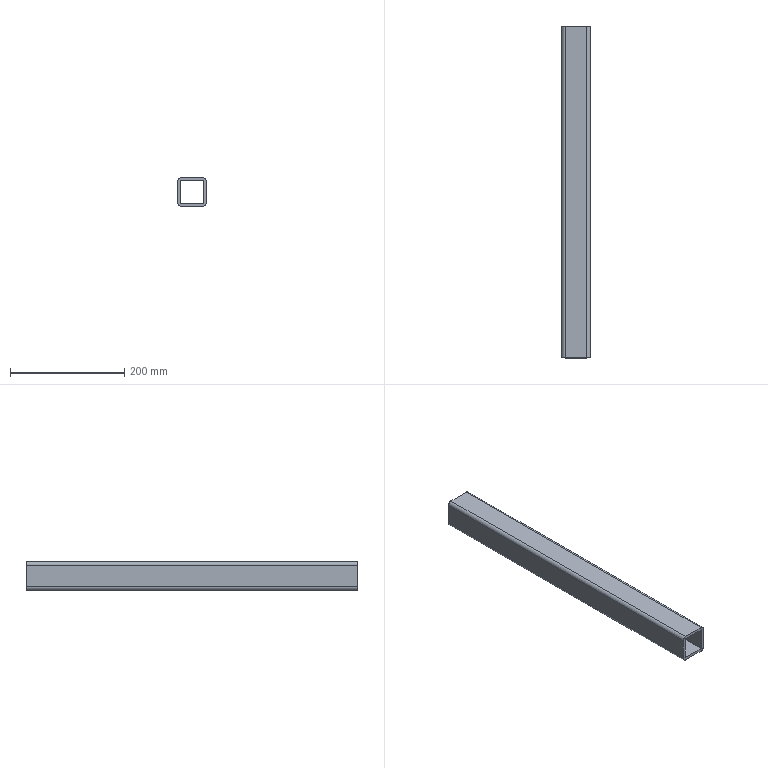Part | SolidWorks | features Extrusion 1 | 1 solid | 18 faces | box 50 x 580 x 50 mm | volume 504574 mm3 | plane 10 | cylinder 8 | commonest cylinder face diameters 2 x4 12 x4
STEP:
#1=CARTESIAN_POINT('',(-25.,580.,6.278));
#2=VERTEX_POINT('',#1);
#3=CARTESIAN_POINT('',(-19.,580.,12.278));
#4=VERTEX_POINT('',#3);
#5=CARTESIAN_POINT('',(-19.,580.,6.278));
#6=DIRECTION('',(0.,1.,0.));
#7=DIRECTION('',(0.,0.,-1.));
#8=AXIS2_PLACEMENT_3D('',#5,#6,#7);
#9=CIRCLE('',#8,6.);
#10=EDGE_CURVE('',#2,#4,#9,.T.);
#11=ORIENTED_EDGE('',*,*,#10,.T.);
#12=CARTESIAN_POINT('',(19.,580.,12.278));
#13=VERTEX_POINT('',#12);
#14=CARTESIAN_POINT('',(-19.,580.,12.278));
#15=DIRECTION('',(1.,0.,0.));
#16=VECTOR('',#15,1000.);
#17=LINE('',#14,#16);
#18=EDGE_CURVE('',#4,#13,#17,.T.);
#19=ORIENTED_EDGE('',*,*,#18,.T.);
#20=CARTESIAN_POINT('',(25.,580.,6.278));
#21=VERTEX_POINT('',#20);
#22=CARTESIAN_POINT('',(19.,580.,6.278));
#23=DIRECTION('',(0.,1.,0.));
#24=DIRECTION('',(0.,0.,1.));
#25=AXIS2_PLACEMENT_3D('',#22,#23,#24);
#26=CIRCLE('',#25,6.);
#27=EDGE_CURVE('',#13,#21,#26,.T.);
#28=ORIENTED_EDGE('',*,*,#27,.T.);
#29=CARTESIAN_POINT('',(25.,580.,-31.722));
#30=VERTEX_POINT('',#29);
#31=CARTESIAN_POINT('',(25.,580.,6.278));
#32=DIRECTION('',(0.,0.,-1.));
#33=VECTOR('',#32,1000.);
#34=LINE('',#31,#33);
#35=EDGE_CURVE('',#21,#30,#34,.T.);
#36=ORIENTED_EDGE('',*,*,#35,.T.);
#37=CARTESIAN_POINT('',(19.,580.,-37.722));
#38=VERTEX_POINT('',#37);
#39=CARTESIAN_POINT('',(19.,580.,-31.722));
#40=DIRECTION('',(0.,1.,0.));
#41=DIRECTION('',(0.,0.,-1.));
#42=AXIS2_PLACEMENT_3D('',#39,#40,#41);
#43=CIRCLE('',#42,6.);
#44=EDGE_CURVE('',#30,#38,#43,.T.);
#45=ORIENTED_EDGE('',*,*,#44,.T.);
#46=CARTESIAN_POINT('',(-19.,580.,-37.722));
#47=VERTEX_POINT('',#46);
#48=CARTESIAN_POINT('',(-19.,580.,-37.722));
#49=DIRECTION('',(-1.,0.,0.));
#50=VECTOR('',#49,1000.);
#51=LINE('',#48,#50);
#52=EDGE_CURVE('',#38,#47,#51,.T.);
#53=ORIENTED_EDGE('',*,*,#52,.T.);
#54=CARTESIAN_POINT('',(-25.,580.,-31.722));
#55=VERTEX_POINT('',#54);
#56=CARTESIAN_POINT('',(-19.,580.,-31.722));
#57=DIRECTION('',(0.,1.,0.));
#58=DIRECTION('',(0.,0.,-1.));
#59=AXIS2_PLACEMENT_3D('',#56,#57,#58);
#60=CIRCLE('',#59,6.);
#61=EDGE_CURVE('',#47,#55,#60,.T.);
#62=ORIENTED_EDGE('',*,*,#61,.T.);
#63=CARTESIAN_POINT('',(-25.,580.,6.278));
#64=DIRECTION('',(0.,0.,1.));
#65=VECTOR('',#64,1000.);
#66=LINE('',#63,#65);
#67=EDGE_CURVE('',#55,#2,#66,.T.);
#68=ORIENTED_EDGE('',*,*,#67,.T.);
#69=EDGE_LOOP('',(#11,#19,#28,#36,#45,#53,#62,#68));
#70=FACE_OUTER_BOUND('',#69,.T.);
#71=CARTESIAN_POINT('',(-20.,580.,6.278));
#72=VERTEX_POINT('',#71);
#73=CARTESIAN_POINT('',(-19.,580.,7.278));
#74=VERTEX_POINT('',#73);
#75=CARTESIAN_POINT('',(-19.,580.,6.278));
#76=DIRECTION('',(0.,1.,0.));
#77=DIRECTION('',(0.,0.,-1.));
#78=AXIS2_PLACEMENT_3D('',#75,#76,#77);
#79=CIRCLE('',#78,1.);
#80=EDGE_CURVE('',#72,#74,#79,.T.);
#81=ORIENTED_EDGE('',*,*,#80,.F.);
#82=CARTESIAN_POINT('',(-20.,580.,-31.722));
#83=VERTEX_POINT('',#82);
#84=CARTESIAN_POINT('',(-20.,580.,6.278));
#85=DIRECTION('',(0.,0.,1.));
#86=VECTOR('',#85,1000.);
#87=LINE('',#84,#86);
#88=EDGE_CURVE('',#83,#72,#87,.T.);
#89=ORIENTED_EDGE('',*,*,#88,.F.);
#90=CARTESIAN_POINT('',(-19.,580.,-32.722));
#91=VERTEX_POINT('',#90);
#92=CARTESIAN_POINT('',(-19.,580.,-31.722));
#93=DIRECTION('',(0.,1.,0.));
#94=DIRECTION('',(0.,0.,-1.));
#95=AXIS2_PLACEMENT_3D('',#92,#93,#94);
#96=CIRCLE('',#95,1.);
#97=EDGE_CURVE('',#91,#83,#96,.T.);
#98=ORIENTED_EDGE('',*,*,#97,.F.);
#99=CARTESIAN_POINT('',(19.,580.,-32.722));
#100=VERTEX_POINT('',#99);
#101=CARTESIAN_POINT('',(-19.,580.,-32.722));
#102=DIRECTION('',(-1.,0.,0.));
#103=VECTOR('',#102,1000.);
#104=LINE('',#101,#103);
#105=EDGE_CURVE('',#100,#91,#104,.T.);
#106=ORIENTED_EDGE('',*,*,#105,.F.);
#107=CARTESIAN_POINT('',(20.,580.,-31.722));
#108=VERTEX_POINT('',#107);
#109=CARTESIAN_POINT('',(19.,580.,-31.722));
#110=DIRECTION('',(0.,1.,0.));
#111=DIRECTION('',(0.,0.,-1.));
#112=AXIS2_PLACEMENT_3D('',#109,#110,#111);
#113=CIRCLE('',#112,1.);
#114=EDGE_CURVE('',#108,#100,#113,.T.);
#115=ORIENTED_EDGE('',*,*,#114,.F.);
#116=CARTESIAN_POINT('',(20.,580.,6.278));
#117=VERTEX_POINT('',#116);
#118=CARTESIAN_POINT('',(20.,580.,6.278));
#119=DIRECTION('',(0.,0.,-1.));
#120=VECTOR('',#119,1000.);
#121=LINE('',#118,#120);
#122=EDGE_CURVE('',#117,#108,#121,.T.);
#123=ORIENTED_EDGE('',*,*,#122,.F.);
#124=CARTESIAN_POINT('',(19.,580.,7.278));
#125=VERTEX_POINT('',#124);
#126=CARTESIAN_POINT('',(19.,580.,6.278));
#127=DIRECTION('',(0.,1.,0.));
#128=DIRECTION('',(0.,0.,1.));
#129=AXIS2_PLACEMENT_3D('',#126,#127,#128);
#130=CIRCLE('',#129,1.);
#131=EDGE_CURVE('',#125,#117,#130,.T.);
#132=ORIENTED_EDGE('',*,*,#131,.F.);
#133=CARTESIAN_POINT('',(-19.,580.,7.278));
#134=DIRECTION('',(1.,0.,0.));
#135=VECTOR('',#134,1000.);
#136=LINE('',#133,#135);
#137=EDGE_CURVE('',#74,#125,#136,.T.);
#138=ORIENTED_EDGE('',*,*,#137,.F.);
#139=EDGE_LOOP('',(#81,#89,#98,#106,#115,#123,#132,#138));
#140=FACE_BOUND('',#139,.T.);
#141=CARTESIAN_POINT('',(-19.,580.,6.278));
#142=DIRECTION('',(0.,-1.,0.));
#143=DIRECTION('',(0.,0.,-1.));
#144=AXIS2_PLACEMENT_3D('',#141,#142,#143);
#145=PLANE('',#144);
#146=ADVANCED_FACE('',(#70,#140),#145,.F.);
#147=CARTESIAN_POINT('',(-25.,0.,6.278));
#148=VERTEX_POINT('',#147);
#149=CARTESIAN_POINT('',(-19.,0.,12.278));
#150=VERTEX_POINT('',#149);
#151=CARTESIAN_POINT('',(-19.,0.,6.278));
#152=DIRECTION('',(0.,1.,0.));
#153=DIRECTION('',(0.,0.,-1.));
#154=AXIS2_PLACEMENT_3D('',#151,#152,#153);
#155=CIRCLE('',#154,6.);
#156=EDGE_CURVE('',#148,#150,#155,.T.);
#157=ORIENTED_EDGE('',*,*,#156,.F.);
#158=CARTESIAN_POINT('',(-25.,0.,-31.722));
#159=VERTEX_POINT('',#158);
#160=CARTESIAN_POINT('',(-25.,0.,6.278));
#161=DIRECTION('',(0.,0.,1.));
#162=VECTOR('',#161,1000.);
#163=LINE('',#160,#162);
#164=EDGE_CURVE('',#159,#148,#163,.T.);
#165=ORIENTED_EDGE('',*,*,#164,.F.);
#166=CARTESIAN_POINT('',(-19.,0.,-37.722));
#167=VERTEX_POINT('',#166);
#168=CARTESIAN_POINT('',(-19.,0.,-31.722));
#169=DIRECTION('',(0.,1.,0.));
#170=DIRECTION('',(0.,0.,-1.));
#171=AXIS2_PLACEMENT_3D('',#168,#169,#170);
#172=CIRCLE('',#171,6.);
#173=EDGE_CURVE('',#167,#159,#172,.T.);
#174=ORIENTED_EDGE('',*,*,#173,.F.);
#175=CARTESIAN_POINT('',(19.,0.,-37.722));
#176=VERTEX_POINT('',#175);
#177=CARTESIAN_POINT('',(-19.,0.,-37.722));
#178=DIRECTION('',(-1.,0.,0.));
#179=VECTOR('',#178,1000.);
#180=LINE('',#177,#179);
#181=EDGE_CURVE('',#176,#167,#180,.T.);
#182=ORIENTED_EDGE('',*,*,#181,.F.);
#183=CARTESIAN_POINT('',(25.,0.,-31.722));
#184=VERTEX_POINT('',#183);
#185=CARTESIAN_POINT('',(19.,0.,-31.722));
#186=DIRECTION('',(0.,1.,0.));
#187=DIRECTION('',(0.,0.,-1.));
#188=AXIS2_PLACEMENT_3D('',#185,#186,#187);
#189=CIRCLE('',#188,6.);
#190=EDGE_CURVE('',#184,#176,#189,.T.);
#191=ORIENTED_EDGE('',*,*,#190,.F.);
#192=CARTESIAN_POINT('',(25.,0.,6.278));
#193=VERTEX_POINT('',#192);
#194=CARTESIAN_POINT('',(25.,0.,6.278));
#195=DIRECTION('',(0.,0.,-1.));
#196=VECTOR('',#195,1000.);
#197=LINE('',#194,#196);
#198=EDGE_CURVE('',#193,#184,#197,.T.);
#199=ORIENTED_EDGE('',*,*,#198,.F.);
#200=CARTESIAN_POINT('',(19.,0.,12.278));
#201=VERTEX_POINT('',#200);
#202=CARTESIAN_POINT('',(19.,0.,6.278));
#203=DIRECTION('',(0.,1.,0.));
#204=DIRECTION('',(0.,0.,1.));
#205=AXIS2_PLACEMENT_3D('',#202,#203,#204);
#206=CIRCLE('',#205,6.);
#207=EDGE_CURVE('',#201,#193,#206,.T.);
#208=ORIENTED_EDGE('',*,*,#207,.F.);
#209=CARTESIAN_POINT('',(-19.,0.,12.278));
#210=DIRECTION('',(1.,0.,0.));
#211=VECTOR('',#210,1000.);
#212=LINE('',#209,#211);
#213=EDGE_CURVE('',#150,#201,#212,.T.);
#214=ORIENTED_EDGE('',*,*,#213,.F.);
#215=EDGE_LOOP('',(#157,#165,#174,#182,#191,#199,#208,#214));
#216=FACE_OUTER_BOUND('',#215,.T.);
#217=CARTESIAN_POINT('',(-20.,0.,-31.722));
#218=VERTEX_POINT('',#217);
#219=CARTESIAN_POINT('',(-20.,0.,6.278));
#220=VERTEX_POINT('',#219);
#221=CARTESIAN_POINT('',(-20.,0.,6.278));
#222=DIRECTION('',(0.,0.,1.));
#223=VECTOR('',#222,1000.);
#224=LINE('',#221,#223);
#225=EDGE_CURVE('',#218,#220,#224,.T.);
#226=ORIENTED_EDGE('',*,*,#225,.T.);
#227=CARTESIAN_POINT('',(-19.,0.,7.278));
#228=VERTEX_POINT('',#227);
#229=CARTESIAN_POINT('',(-19.,0.,6.278));
#230=DIRECTION('',(0.,1.,0.));
#231=DIRECTION('',(0.,0.,-1.));
#232=AXIS2_PLACEMENT_3D('',#229,#230,#231);
#233=CIRCLE('',#232,1.);
#234=EDGE_CURVE('',#220,#228,#233,.T.);
#235=ORIENTED_EDGE('',*,*,#234,.T.);
#236=CARTESIAN_POINT('',(19.,0.,7.278));
#237=VERTEX_POINT('',#236);
#238=CARTESIAN_POINT('',(-19.,0.,7.278));
#239=DIRECTION('',(1.,0.,0.));
#240=VECTOR('',#239,1000.);
#241=LINE('',#238,#240);
#242=EDGE_CURVE('',#228,#237,#241,.T.);
#243=ORIENTED_EDGE('',*,*,#242,.T.);
#244=CARTESIAN_POINT('',(20.,0.,6.278));
#245=VERTEX_POINT('',#244);
#246=CARTESIAN_POINT('',(19.,0.,6.278));
#247=DIRECTION('',(0.,1.,0.));
#248=DIRECTION('',(0.,0.,1.));
#249=AXIS2_PLACEMENT_3D('',#246,#247,#248);
#250=CIRCLE('',#249,1.);
#251=EDGE_CURVE('',#237,#245,#250,.T.);
#252=ORIENTED_EDGE('',*,*,#251,.T.);
#253=CARTESIAN_POINT('',(20.,0.,-31.722));
#254=VERTEX_POINT('',#253);
#255=CARTESIAN_POINT('',(20.,0.,6.278));
#256=DIRECTION('',(0.,0.,-1.));
#257=VECTOR('',#256,1000.);
#258=LINE('',#255,#257);
#259=EDGE_CURVE('',#245,#254,#258,.T.);
#260=ORIENTED_EDGE('',*,*,#259,.T.);
#261=CARTESIAN_POINT('',(19.,0.,-32.722));
#262=VERTEX_POINT('',#261);
#263=CARTESIAN_POINT('',(19.,0.,-31.722));
#264=DIRECTION('',(0.,1.,0.));
#265=DIRECTION('',(0.,0.,-1.));
#266=AXIS2_PLACEMENT_3D('',#263,#264,#265);
#267=CIRCLE('',#266,1.);
#268=EDGE_CURVE('',#254,#262,#267,.T.);
#269=ORIENTED_EDGE('',*,*,#268,.T.);
#270=CARTESIAN_POINT('',(-19.,0.,-32.722));
#271=VERTEX_POINT('',#270);
#272=CARTESIAN_POINT('',(-19.,0.,-32.722));
#273=DIRECTION('',(-1.,0.,0.));
#274=VECTOR('',#273,1000.);
#275=LINE('',#272,#274);
#276=EDGE_CURVE('',#262,#271,#275,.T.);
#277=ORIENTED_EDGE('',*,*,#276,.T.);
#278=CARTESIAN_POINT('',(-19.,0.,-31.722));
#279=DIRECTION('',(0.,1.,0.));
#280=DIRECTION('',(0.,0.,-1.));
#281=AXIS2_PLACEMENT_3D('',#278,#279,#280);
#282=CIRCLE('',#281,1.);
#283=EDGE_CURVE('',#271,#218,#282,.T.);
#284=ORIENTED_EDGE('',*,*,#283,.T.);
#285=EDGE_LOOP('',(#226,#235,#243,#252,#260,#269,#277,#284));
#286=FACE_BOUND('',#285,.T.);
#287=CARTESIAN_POINT('',(-19.,0.,6.278));
#288=DIRECTION('',(0.,-1.,0.));
#289=DIRECTION('',(0.,0.,-1.));
#290=AXIS2_PLACEMENT_3D('',#287,#288,#289);
#291=PLANE('',#290);
#292=ADVANCED_FACE('',(#216,#286),#291,.T.);
#293=ORIENTED_EDGE('',*,*,#156,.T.);
#294=CARTESIAN_POINT('',(-19.,580.,12.278));
#295=DIRECTION('',(0.,-1.,0.));
#296=VECTOR('',#295,1000.);
#297=LINE('',#294,#296);
#298=EDGE_CURVE('',#4,#150,#297,.T.);
#299=ORIENTED_EDGE('',*,*,#298,.F.);
#300=ORIENTED_EDGE('',*,*,#10,.F.);
#301=CARTESIAN_POINT('',(-25.,580.,6.278));
#302=DIRECTION('',(0.,-1.,0.));
#303=VECTOR('',#302,1000.);
#304=LINE('',#301,#303);
#305=EDGE_CURVE('',#2,#148,#304,.T.);
#306=ORIENTED_EDGE('',*,*,#305,.T.);
#307=EDGE_LOOP('',(#293,#299,#300,#306));
#308=FACE_OUTER_BOUND('',#307,.T.);
#309=CARTESIAN_POINT('',(-19.,580.,6.278));
#310=DIRECTION('',(0.,-1.,0.));
#311=DIRECTION('',(0.,0.,-1.));
#312=AXIS2_PLACEMENT_3D('',#309,#310,#311);
#313=CYLINDRICAL_SURFACE('',#312,6.);
#314=ADVANCED_FACE('',(#308),#313,.T.);
#315=ORIENTED_EDGE('',*,*,#213,.T.);
#316=CARTESIAN_POINT('',(19.,580.,12.278));
#317=DIRECTION('',(0.,-1.,0.));
#318=VECTOR('',#317,1000.);
#319=LINE('',#316,#318);
#320=EDGE_CURVE('',#13,#201,#319,.T.);
#321=ORIENTED_EDGE('',*,*,#320,.F.);
#322=ORIENTED_EDGE('',*,*,#18,.F.);
#323=ORIENTED_EDGE('',*,*,#298,.T.);
#324=EDGE_LOOP('',(#315,#321,#322,#323));
#325=FACE_OUTER_BOUND('',#324,.T.);
#326=CARTESIAN_POINT('',(-19.,580.,12.278));
#327=DIRECTION('',(0.,0.,-1.));
#328=DIRECTION('',(-1.,0.,0.));
#329=AXIS2_PLACEMENT_3D('',#326,#327,#328);
#330=PLANE('',#329);
#331=ADVANCED_FACE('',(#325),#330,.F.);
#332=ORIENTED_EDGE('',*,*,#207,.T.);
#333=CARTESIAN_POINT('',(25.,580.,6.278));
#334=DIRECTION('',(0.,-1.,0.));
#335=VECTOR('',#334,1000.);
#336=LINE('',#333,#335);
#337=EDGE_CURVE('',#21,#193,#336,.T.);
#338=ORIENTED_EDGE('',*,*,#337,.F.);
#339=ORIENTED_EDGE('',*,*,#27,.F.);
#340=ORIENTED_EDGE('',*,*,#320,.T.);
#341=EDGE_LOOP('',(#332,#338,#339,#340));
#342=FACE_OUTER_BOUND('',#341,.T.);
#343=CARTESIAN_POINT('',(19.,580.,6.278));
#344=DIRECTION('',(0.,-1.,0.));
#345=DIRECTION('',(0.,0.,-1.));
#346=AXIS2_PLACEMENT_3D('',#343,#344,#345);
#347=CYLINDRICAL_SURFACE('',#346,6.);
#348=ADVANCED_FACE('',(#342),#347,.T.);
#349=ORIENTED_EDGE('',*,*,#198,.T.);
#350=CARTESIAN_POINT('',(25.,580.,-31.722));
#351=DIRECTION('',(0.,-1.,0.));
#352=VECTOR('',#351,1000.);
#353=LINE('',#350,#352);
#354=EDGE_CURVE('',#30,#184,#353,.T.);
#355=ORIENTED_EDGE('',*,*,#354,.F.);
#356=ORIENTED_EDGE('',*,*,#35,.F.);
#357=ORIENTED_EDGE('',*,*,#337,.T.);
#358=EDGE_LOOP('',(#349,#355,#356,#357));
#359=FACE_OUTER_BOUND('',#358,.T.);
#360=CARTESIAN_POINT('',(25.,580.,6.278));
#361=DIRECTION('',(-1.,0.,0.));
#362=DIRECTION('',(0.,0.,1.));
#363=AXIS2_PLACEMENT_3D('',#360,#361,#362);
#364=PLANE('',#363);
#365=ADVANCED_FACE('',(#359),#364,.F.);
#366=ORIENTED_EDGE('',*,*,#190,.T.);
#367=CARTESIAN_POINT('',(19.,580.,-37.722));
#368=DIRECTION('',(0.,-1.,0.));
#369=VECTOR('',#368,1000.);
#370=LINE('',#367,#369);
#371=EDGE_CURVE('',#38,#176,#370,.T.);
#372=ORIENTED_EDGE('',*,*,#371,.F.);
#373=ORIENTED_EDGE('',*,*,#44,.F.);
#374=ORIENTED_EDGE('',*,*,#354,.T.);
#375=EDGE_LOOP('',(#366,#372,#373,#374));
#376=FACE_OUTER_BOUND('',#375,.T.);
#377=CARTESIAN_POINT('',(19.,580.,-31.722));
#378=DIRECTION('',(0.,-1.,0.));
#379=DIRECTION('',(0.,0.,-1.));
#380=AXIS2_PLACEMENT_3D('',#377,#378,#379);
#381=CYLINDRICAL_SURFACE('',#380,6.);
#382=ADVANCED_FACE('',(#376),#381,.T.);
#383=ORIENTED_EDGE('',*,*,#181,.T.);
#384=CARTESIAN_POINT('',(-19.,580.,-37.722));
#385=DIRECTION('',(0.,-1.,0.));
#386=VECTOR('',#385,1000.);
#387=LINE('',#384,#386);
#388=EDGE_CURVE('',#47,#167,#387,.T.);
#389=ORIENTED_EDGE('',*,*,#388,.F.);
#390=ORIENTED_EDGE('',*,*,#52,.F.);
#391=ORIENTED_EDGE('',*,*,#371,.T.);
#392=EDGE_LOOP('',(#383,#389,#390,#391));
#393=FACE_OUTER_BOUND('',#392,.T.);
#394=CARTESIAN_POINT('',(-19.,580.,-37.722));
#395=DIRECTION('',(0.,0.,1.));
#396=DIRECTION('',(1.,0.,0.));
#397=AXIS2_PLACEMENT_3D('',#394,#395,#396);
#398=PLANE('',#397);
#399=ADVANCED_FACE('',(#393),#398,.F.);
#400=ORIENTED_EDGE('',*,*,#173,.T.);
#401=CARTESIAN_POINT('',(-25.,580.,-31.722));
#402=DIRECTION('',(0.,-1.,0.));
#403=VECTOR('',#402,1000.);
#404=LINE('',#401,#403);
#405=EDGE_CURVE('',#55,#159,#404,.T.);
#406=ORIENTED_EDGE('',*,*,#405,.F.);
#407=ORIENTED_EDGE('',*,*,#61,.F.);
#408=ORIENTED_EDGE('',*,*,#388,.T.);
#409=EDGE_LOOP('',(#400,#406,#407,#408));
#410=FACE_OUTER_BOUND('',#409,.T.);
#411=CARTESIAN_POINT('',(-19.,580.,-31.722));
#412=DIRECTION('',(0.,-1.,0.));
#413=DIRECTION('',(0.,0.,-1.));
#414=AXIS2_PLACEMENT_3D('',#411,#412,#413);
#415=CYLINDRICAL_SURFACE('',#414,6.);
#416=ADVANCED_FACE('',(#410),#415,.T.);
#417=ORIENTED_EDGE('',*,*,#164,.T.);
#418=ORIENTED_EDGE('',*,*,#305,.F.);
#419=ORIENTED_EDGE('',*,*,#67,.F.);
#420=ORIENTED_EDGE('',*,*,#405,.T.);
#421=EDGE_LOOP('',(#417,#418,#419,#420));
#422=FACE_OUTER_BOUND('',#421,.T.);
#423=CARTESIAN_POINT('',(-25.,580.,6.278));
#424=DIRECTION('',(1.,0.,0.));
#425=DIRECTION('',(0.,0.,-1.));
#426=AXIS2_PLACEMENT_3D('',#423,#424,#425);
#427=PLANE('',#426);
#428=ADVANCED_FACE('',(#422),#427,.F.);
#429=ORIENTED_EDGE('',*,*,#234,.F.);
#430=CARTESIAN_POINT('',(-20.,580.,6.278));
#431=DIRECTION('',(0.,-1.,0.));
#432=VECTOR('',#431,1000.);
#433=LINE('',#430,#432);
#434=EDGE_CURVE('',#72,#220,#433,.T.);
#435=ORIENTED_EDGE('',*,*,#434,.F.);
#436=ORIENTED_EDGE('',*,*,#80,.T.);
#437=CARTESIAN_POINT('',(-19.,580.,7.278));
#438=DIRECTION('',(0.,-1.,0.));
#439=VECTOR('',#438,1000.);
#440=LINE('',#437,#439);
#441=EDGE_CURVE('',#74,#228,#440,.T.);
#442=ORIENTED_EDGE('',*,*,#441,.T.);
#443=EDGE_LOOP('',(#429,#435,#436,#442));
#444=FACE_OUTER_BOUND('',#443,.T.);
#445=CARTESIAN_POINT('',(-19.,580.,6.278));
#446=DIRECTION('',(0.,-1.,0.));
#447=DIRECTION('',(0.,0.,-1.));
#448=AXIS2_PLACEMENT_3D('',#445,#446,#447);
#449=CYLINDRICAL_SURFACE('',#448,1.);
#450=ADVANCED_FACE('',(#444),#449,.F.);
#451=ORIENTED_EDGE('',*,*,#242,.F.);
#452=ORIENTED_EDGE('',*,*,#441,.F.);
#453=ORIENTED_EDGE('',*,*,#137,.T.);
#454=CARTESIAN_POINT('',(19.,580.,7.278));
#455=DIRECTION('',(0.,-1.,0.));
#456=VECTOR('',#455,1000.);
#457=LINE('',#454,#456);
#458=EDGE_CURVE('',#125,#237,#457,.T.);
#459=ORIENTED_EDGE('',*,*,#458,.T.);
#460=EDGE_LOOP('',(#451,#452,#453,#459));
#461=FACE_OUTER_BOUND('',#460,.T.);
#462=CARTESIAN_POINT('',(-19.,580.,7.278));
#463=DIRECTION('',(0.,0.,-1.));
#464=DIRECTION('',(-1.,0.,0.));
#465=AXIS2_PLACEMENT_3D('',#462,#463,#464);
#466=PLANE('',#465);
#467=ADVANCED_FACE('',(#461),#466,.T.);
#468=ORIENTED_EDGE('',*,*,#251,.F.);
#469=ORIENTED_EDGE('',*,*,#458,.F.);
#470=ORIENTED_EDGE('',*,*,#131,.T.);
#471=CARTESIAN_POINT('',(20.,580.,6.278));
#472=DIRECTION('',(0.,-1.,0.));
#473=VECTOR('',#472,1000.);
#474=LINE('',#471,#473);
#475=EDGE_CURVE('',#117,#245,#474,.T.);
#476=ORIENTED_EDGE('',*,*,#475,.T.);
#477=EDGE_LOOP('',(#468,#469,#470,#476));
#478=FACE_OUTER_BOUND('',#477,.T.);
#479=CARTESIAN_POINT('',(19.,580.,6.278));
#480=DIRECTION('',(0.,-1.,0.));
#481=DIRECTION('',(0.,0.,-1.));
#482=AXIS2_PLACEMENT_3D('',#479,#480,#481);
#483=CYLINDRICAL_SURFACE('',#482,1.);
#484=ADVANCED_FACE('',(#478),#483,.F.);
#485=ORIENTED_EDGE('',*,*,#259,.F.);
#486=ORIENTED_EDGE('',*,*,#475,.F.);
#487=ORIENTED_EDGE('',*,*,#122,.T.);
#488=CARTESIAN_POINT('',(20.,580.,-31.722));
#489=DIRECTION('',(0.,-1.,0.));
#490=VECTOR('',#489,1000.);
#491=LINE('',#488,#490);
#492=EDGE_CURVE('',#108,#254,#491,.T.);
#493=ORIENTED_EDGE('',*,*,#492,.T.);
#494=EDGE_LOOP('',(#485,#486,#487,#493));
#495=FACE_OUTER_BOUND('',#494,.T.);
#496=CARTESIAN_POINT('',(20.,580.,6.278));
#497=DIRECTION('',(-1.,0.,0.));
#498=DIRECTION('',(0.,0.,1.));
#499=AXIS2_PLACEMENT_3D('',#496,#497,#498);
#500=PLANE('',#499);
#501=ADVANCED_FACE('',(#495),#500,.T.);
#502=ORIENTED_EDGE('',*,*,#268,.F.);
#503=ORIENTED_EDGE('',*,*,#492,.F.);
#504=ORIENTED_EDGE('',*,*,#114,.T.);
#505=CARTESIAN_POINT('',(19.,580.,-32.722));
#506=DIRECTION('',(0.,-1.,0.));
#507=VECTOR('',#506,1000.);
#508=LINE('',#505,#507);
#509=EDGE_CURVE('',#100,#262,#508,.T.);
#510=ORIENTED_EDGE('',*,*,#509,.T.);
#511=EDGE_LOOP('',(#502,#503,#504,#510));
#512=FACE_OUTER_BOUND('',#511,.T.);
#513=CARTESIAN_POINT('',(19.,580.,-31.722));
#514=DIRECTION('',(0.,-1.,0.));
#515=DIRECTION('',(0.,0.,-1.));
#516=AXIS2_PLACEMENT_3D('',#513,#514,#515);
#517=CYLINDRICAL_SURFACE('',#516,1.);
#518=ADVANCED_FACE('',(#512),#517,.F.);
#519=ORIENTED_EDGE('',*,*,#276,.F.);
#520=ORIENTED_EDGE('',*,*,#509,.F.);
#521=ORIENTED_EDGE('',*,*,#105,.T.);
#522=CARTESIAN_POINT('',(-19.,580.,-32.722));
#523=DIRECTION('',(0.,-1.,0.));
#524=VECTOR('',#523,1000.);
#525=LINE('',#522,#524);
#526=EDGE_CURVE('',#91,#271,#525,.T.);
#527=ORIENTED_EDGE('',*,*,#526,.T.);
#528=EDGE_LOOP('',(#519,#520,#521,#527));
#529=FACE_OUTER_BOUND('',#528,.T.);
#530=CARTESIAN_POINT('',(-19.,580.,-32.722));
#531=DIRECTION('',(0.,0.,1.));
#532=DIRECTION('',(1.,0.,0.));
#533=AXIS2_PLACEMENT_3D('',#530,#531,#532);
#534=PLANE('',#533);
#535=ADVANCED_FACE('',(#529),#534,.T.);
#536=ORIENTED_EDGE('',*,*,#283,.F.);
#537=ORIENTED_EDGE('',*,*,#526,.F.);
#538=ORIENTED_EDGE('',*,*,#97,.T.);
#539=CARTESIAN_POINT('',(-20.,580.,-31.722));
#540=DIRECTION('',(0.,-1.,0.));
#541=VECTOR('',#540,1000.);
#542=LINE('',#539,#541);
#543=EDGE_CURVE('',#83,#218,#542,.T.);
#544=ORIENTED_EDGE('',*,*,#543,.T.);
#545=EDGE_LOOP('',(#536,#537,#538,#544));
#546=FACE_OUTER_BOUND('',#545,.T.);
#547=CARTESIAN_POINT('',(-19.,580.,-31.722));
#548=DIRECTION('',(0.,-1.,0.));
#549=DIRECTION('',(0.,0.,-1.));
#550=AXIS2_PLACEMENT_3D('',#547,#548,#549);
#551=CYLINDRICAL_SURFACE('',#550,1.);
#552=ADVANCED_FACE('',(#546),#551,.F.);
#553=ORIENTED_EDGE('',*,*,#225,.F.);
#554=ORIENTED_EDGE('',*,*,#543,.F.);
#555=ORIENTED_EDGE('',*,*,#88,.T.);
#556=ORIENTED_EDGE('',*,*,#434,.T.);
#557=EDGE_LOOP('',(#553,#554,#555,#556));
#558=FACE_OUTER_BOUND('',#557,.T.);
#559=CARTESIAN_POINT('',(-20.,580.,6.278));
#560=DIRECTION('',(1.,0.,0.));
#561=DIRECTION('',(0.,0.,-1.));
#562=AXIS2_PLACEMENT_3D('',#559,#560,#561);
#563=PLANE('',#562);
#564=ADVANCED_FACE('',(#558),#563,.T.);
#565=CLOSED_SHELL('',(#146,#292,#314,#331,#348,#365,#382,#399,#416,#428,#450,#467,#484,#501,#518,#535,#552,#564));
#566=MANIFOLD_SOLID_BREP('',#565);
#567=CARTESIAN_POINT('',(0.,0.,0.));
#568=DIRECTION('',(0.,0.,1.));
#569=DIRECTION('',(1.,0.,0.));
#570=AXIS2_PLACEMENT_3D('',#567,#568,#569);
#571=(LENGTH_UNIT()NAMED_UNIT(*)SI_UNIT(.MILLI.,.METRE.));
#572=UNCERTAINTY_MEASURE_WITH_UNIT(LENGTH_MEASURE(0.00001),#571,'','');
#573=(NAMED_UNIT(*)PLANE_ANGLE_UNIT()SI_UNIT($,.RADIAN.));
#574=(NAMED_UNIT(*)SI_UNIT($,.STERADIAN.)SOLID_ANGLE_UNIT());
#575=(GEOMETRIC_REPRESENTATION_CONTEXT(3)GLOBAL_UNCERTAINTY_ASSIGNED_CONTEXT((#572))GLOBAL_UNIT_ASSIGNED_CONTEXT((#571,#573,#574))REPRESENTATION_CONTEXT('',''));
#576=ADVANCED_BREP_SHAPE_REPRESENTATION('',(#566,#570),#575);